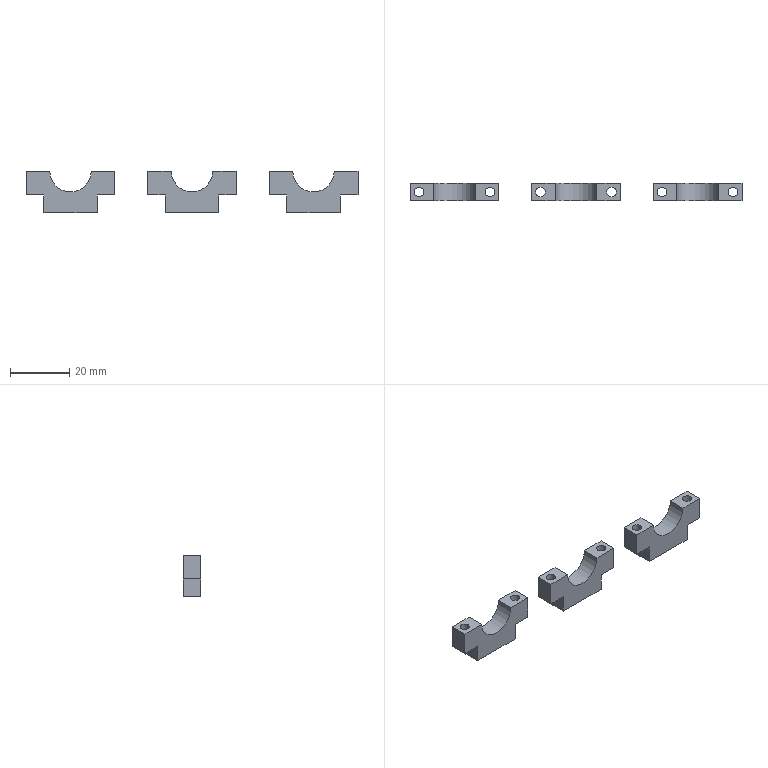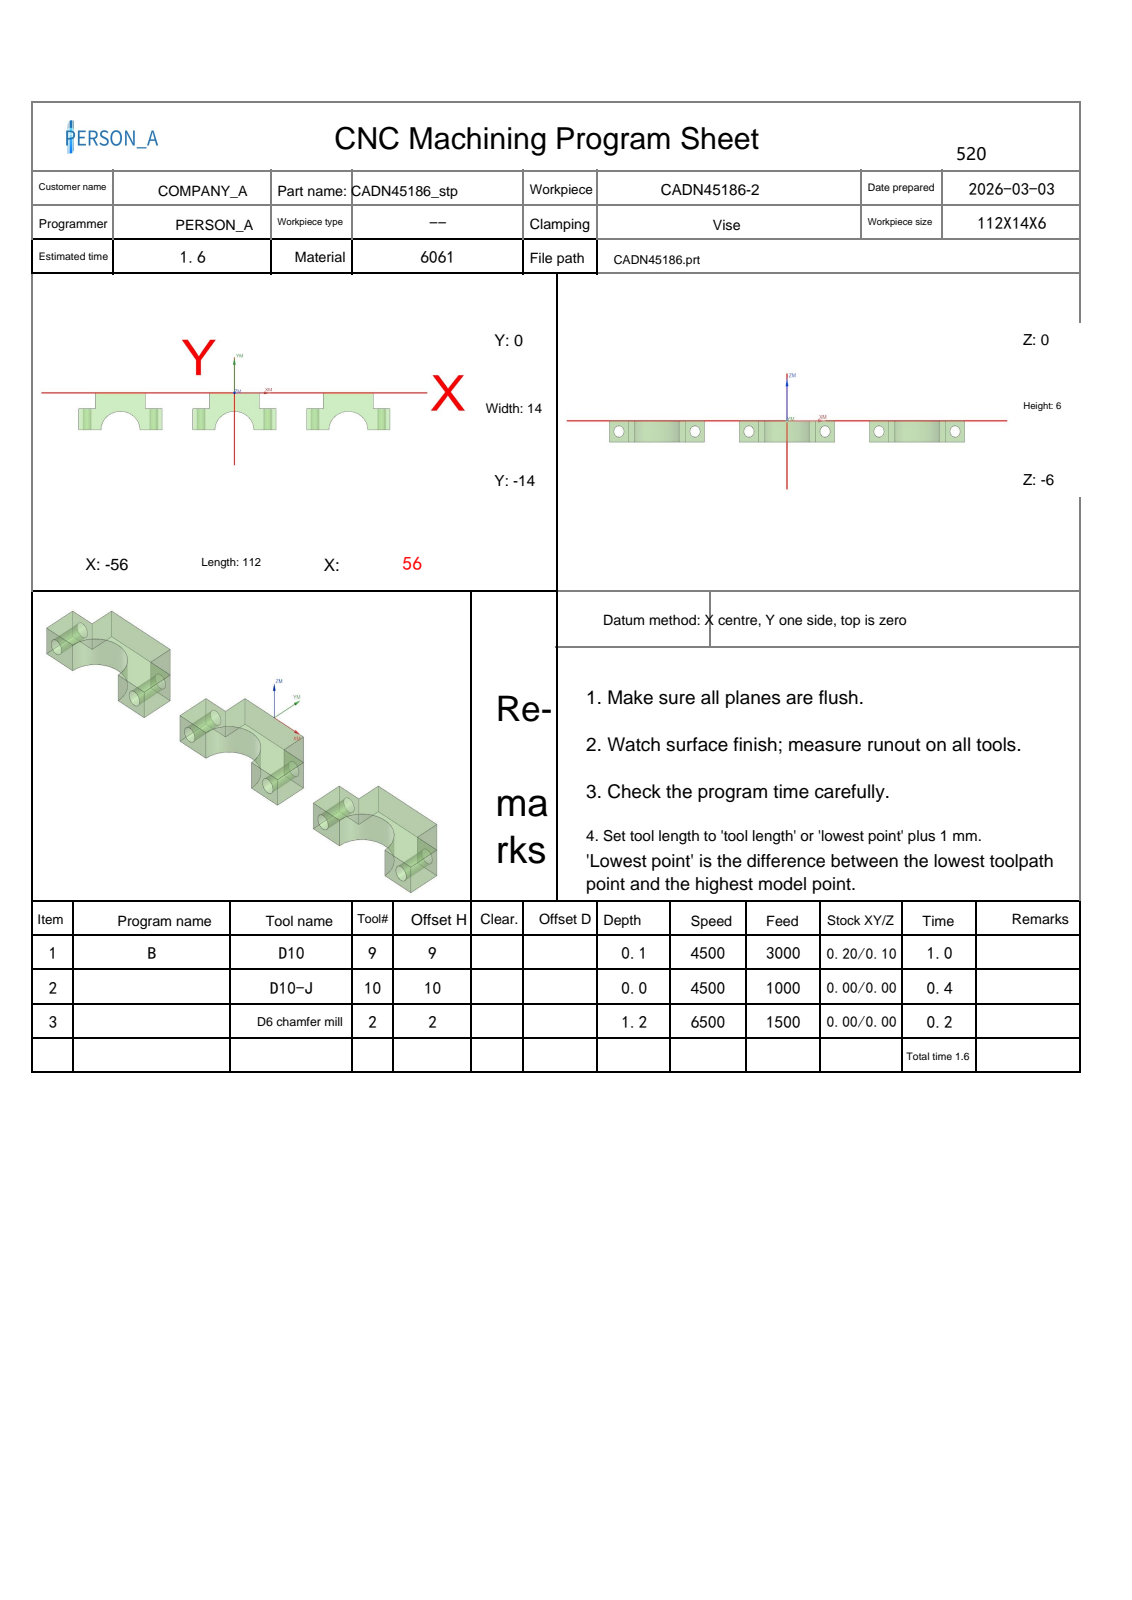NC program | NX | posted by the shop | part box 112 x 6 x 14 mm
Whole program:
%
O0001
(Machine time: 2.26 MIN)
(===Total Tool:3===)
(T9=D10     D=10.  R=0.   D-  H09 Z=0.1   )
(T10=D10-J  D=10.  R=0.   D-  H10 Z=0.    )
(T2=D6 chamfer mill   D=6.   R=0.   D-  H02 Z=-1.2  )
G80 G90 G17 G49 G40
G91 G28 Z0
M01
N1 T09 M06
(D10  D=10. R=0. H=09 ce=0.20 di=0.10)
(MAX_Z=50. MIN_Z=0.1 Time=1.02M)
G00 G90 G54 X73. Y-13. M03 S4500
G43 H09 Z50.
M08
Z5.014
G01 Z3.014 F3000.
X61.
X-60.1
G02 X-61. Y-12.1 I0.0 J.9
G01 Y-7.9
G02 X-60.1 Y-7. I.9 J0.0
G01 X60.1
G03 X61. Y-6.1 I0.0 J.9
G01 Y-1.9
G03 X60.1 Y-1. I-.9 J0.0
G01 X-61.
X-73.
Z5.014
G00 Z6.5
X73. Y-13.
Z4.529
G01 Z2.529
X61.
X-60.1
G02 X-61. Y-12.1 I0.0 J.9
G01 Y-7.9
G02 X-60.1 Y-7. I.9 J0.0
G01 X60.1
G03 X61. Y-6.1 I0.0 J.9
G01 Y-1.9
G03 X60.1 Y-1. I-.9 J0.0
G01 X-61.
X-73.
Z4.529
G00 Z6.014
X73. Y-13.
Z4.043
G01 Z2.043
X61.
X-60.1
G02 X-61. Y-12.1 I0.0 J.9
G01 Y-7.9
G02 X-60.1 Y-7. I.9 J0.0
G01 X60.1
G03 X61. Y-6.1 I0.0 J.9
G01 Y-1.9
G03 X60.1 Y-1. I-.9 J0.0
G01 X-61.
X-73.
Z4.043
G00 Z5.529
X73. Y-13.
Z3.557
G01 Z1.557
X61.
X-60.1
G02 X-61. Y-12.1 I0.0 J.9
G01 Y-7.9
G02 X-60.1 Y-7. I.9 J0.0
G01 X60.1
G03 X61. Y-6.1 I0.0 J.9
G01 Y-1.9
G03 X60.1 Y-1. I-.9 J0.0
G01 X-61.
X-73.
Z3.557
G00 Z5.043
X73. Y-13.
Z3.071
G01 Z1.071
X61.
X-60.1
G02 X-61. Y-12.1 I0.0 J.9
G01 Y-7.9
G02 X-60.1 Y-7. I.9 J0.0
G01 X60.1
G03 X61. Y-6.1 I0.0 J.9
G01 Y-1.9
G03 X60.1 Y-1. I-.9 J0.0
G01 X-61.
X-73.
Z3.071
G00 Z4.557
X73. Y-13.
Z2.586
G01 Z.586
X61.
X-60.1
G02 X-61. Y-12.1 I0.0 J.9
G01 Y-7.9
G02 X-60.1 Y-7. I.9 J0.0
G01 X60.1
G03 X61. Y-6.1 I0.0 J.9
G01 Y-1.9
G03 X60.1 Y-1. I-.9 J0.0
G01 X-61.
X-73.
Z2.586
G00 Z4.071
X73. Y-13.
Z2.1
G01 Z.1
X61.
X-60.1
G02 X-61. Y-12.1 I0.0 J.9
G01 Y-7.9
G02 X-60.1 Y-7. I.9 J0.0
G01 X60.1
G03 X61. Y-6.1 I0.0 J.9
G01 Y-1.9
G03 X60.1 Y-1. I-.9 J0.0
G01 X-61.
X-73.
Z2.1
G00 Z50.
G91 G28 Z0.0
M05
M09
G91 G28 Z0.0
M01
N2 T10 M06
(D10-J  D=10. R=0. H=10 ce=0.00 di=0.00)
(MAX_Z=50. MIN_Z=0. Time=0.42M)
G00 G90 G54 X73. Y-13. M03 S4500
G43 H10 Z50.
M08
Z2.
G01 Z0.0 F1000.
X61.
X-61.
Y-7.
X61.
Y-1.
X-61.
X-73.
Z2.
G00 Z50.
G91 G28 Z0.0
M05
M09
G91 G28 Z0.0
M01
N3 T02 M06
(D6 chamfer mill  D=6. R=0. H=02 ce=0.00 di=0.00)
(MAX_Z=50. MIN_Z=-1.2 Time=0.23M)
G00 G90 G54 X-41.386 Y1.227 M03 S6500
G43 H02 Z50.
M08
Z.172
G01 Z-1.2 F1500.
G03 X-41.1 Y1.027 I1.286 J1.532
G01 X-41.054 Y.997
X-41. Y1.
X-32.
G02 X-31. Y0.0 I0.0 J-1.
G01 Y-5.
X-26.
G02 X-25. Y-6. I0.0 J-1.
G01 Y-14.
G02 X-26. Y-15. I-1. J0.0
G01 X-34.
G02 X-35. Y-14. I0.0 J1.
G03 X-41. Y-8. I-6. J0.0
X-47. Y-14. I0.0 J-6.
G02 X-48. Y-15. I-1. J0.0
G01 X-56.
G02 X-57. Y-14. I0.0 J1.
G01 Y-6.
G02 X-56. Y-5. I1. J0.0
G01 X-51.
Y0.0
G02 X-50. Y1. I1. J0.0
G01 X-41.
X-40.946 Y.997
X-40.9 Y1.027
G03 X-40.614 Y1.227 I-1. J1.732
G01 Z.172
G00 Z10.
X-.386
Z.172
G01 Z-1.2
G03 X-.1 Y1.027 I1.286 J1.532
G01 X-.054 Y.997
X0.0 Y1.
X9.
G02 X10. Y0.0 I0.0 J-1.
G01 Y-5.
X15.
G02 X16. Y-6. I0.0 J-1.
G01 Y-14.
G02 X15. Y-15. I-1. J0.0
G01 X7.
G02 X6. Y-14. I0.0 J1.
G03 X0.0 Y-8. I-6. J0.0
X-6. Y-14. I0.0 J-6.
G02 X-7. Y-15. I-1. J0.0
G01 X-15.
G02 X-16. Y-14. I0.0 J1.
G01 Y-6.
G02 X-15. Y-5. I1. J0.0
G01 X-10.
Y0.0
G02 X-9. Y1. I1. J0.0
G01 X0.0
X.054 Y.997
X.1 Y1.027
G03 X.386 Y1.227 I-1. J1.732
G01 Z.172
G00 Z10.
X40.614
Z.172
G01 Z-1.2
G03 X40.9 Y1.027 I1.286 J1.532
G01 X40.946 Y.997
X41. Y1.
X50.
G02 X51. Y0.0 I0.0 J-1.
G01 Y-5.
X56.
G02 X57. Y-6. I0.0 J-1.
G01 Y-14.
G02 X56. Y-15. I-1. J0.0
G01 X48.
G02 X47. Y-14. I0.0 J1.
G03 X41. Y-8. I-6. J0.0
X35. Y-14. I0.0 J-6.
G02 X34. Y-15. I-1. J0.0
G01 X26.
G02 X25. Y-14. I0.0 J1.
G01 Y-6.
G02 X26. Y-5. I1. J0.0
G01 X31.
Y0.0
G02 X32. Y1. I1. J0.0
G01 X41.
X41.054 Y.997
X41.1 Y1.027
G03 X41.386 Y1.227 I-1. J1.732
G01 Z.172
G00 Z50.
M05
M09
G91 G28 Z0.0
G91 G28 Y0.0
M30
%